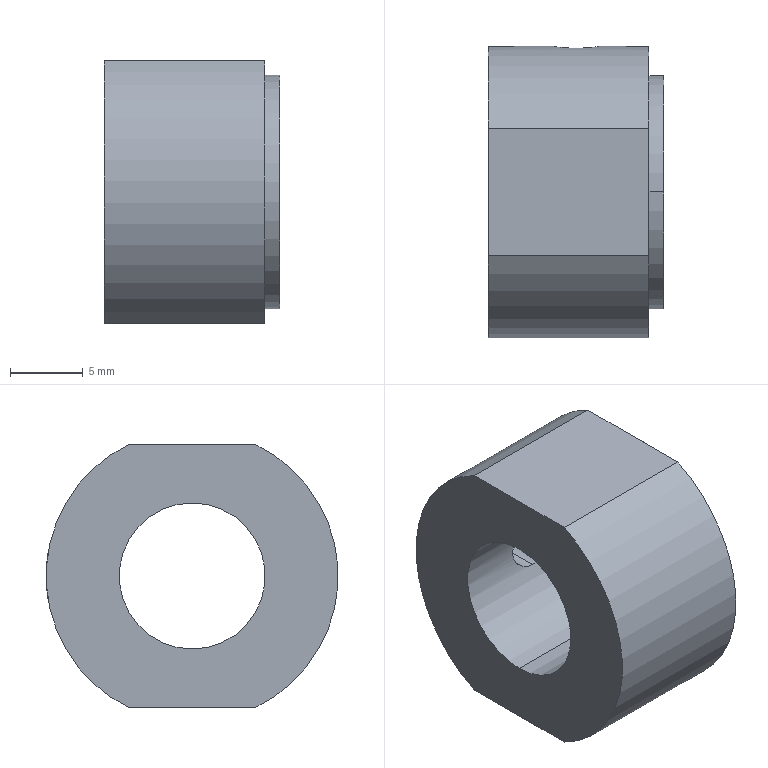Part | SolidWorks | features HoleWzd 1, ICE 1, Revolution 1 | 1 solid | 13 faces | box 12 x 20 x 18 mm | volume 2542 mm3 | cylinder 8 | plane 5 | commonest cylinder face diameters 3.3 x2 10 x2 16 x2 20 x2
STEP:
#1=CARTESIAN_POINT('',(6.,4.72,-1.65));
#2=VERTEX_POINT('',#1);
#3=CARTESIAN_POINT('',(6.,4.72,1.65));
#4=VERTEX_POINT('',#3);
#5=CARTESIAN_POINT('',(6.,4.72,-1.65));
#6=CARTESIAN_POINT('',(5.784,4.72,-1.65));
#7=CARTESIAN_POINT('',(5.565,4.736,-1.606));
#8=CARTESIAN_POINT('',(5.267,4.776,-1.482));
#9=CARTESIAN_POINT('',(5.17,4.791,-1.43));
#10=CARTESIAN_POINT('',(4.992,4.826,-1.311));
#11=CARTESIAN_POINT('',(4.91,4.844,-1.243));
#12=CARTESIAN_POINT('',(4.681,4.899,-1.014));
#13=CARTESIAN_POINT('',(4.56,4.934,-0.8345));
#14=CARTESIAN_POINT('',(4.435,4.972,-0.5335));
#15=CARTESIAN_POINT('',(4.403,4.983,-0.4304));
#16=CARTESIAN_POINT('',(4.361,4.996,-0.2186));
#17=CARTESIAN_POINT('',(4.35,5.,-0.1085));
#18=CARTESIAN_POINT('',(4.35,5.,0.1089));
#19=CARTESIAN_POINT('',(4.361,4.996,0.2166));
#20=CARTESIAN_POINT('',(4.403,4.983,0.4298));
#21=CARTESIAN_POINT('',(4.435,4.972,0.5348));
#22=CARTESIAN_POINT('',(4.559,4.934,0.8329));
#23=CARTESIAN_POINT('',(4.682,4.898,1.016));
#24=CARTESIAN_POINT('',(4.909,4.844,1.242));
#25=CARTESIAN_POINT('',(4.993,4.825,1.312));
#26=CARTESIAN_POINT('',(5.172,4.791,1.431));
#27=CARTESIAN_POINT('',(5.266,4.776,1.482));
#28=CARTESIAN_POINT('',(5.465,4.749,1.565));
#29=CARTESIAN_POINT('',(5.57,4.738,1.597));
#30=CARTESIAN_POINT('',(5.782,4.724,1.639));
#31=CARTESIAN_POINT('',(5.89,4.72,1.65));
#32=CARTESIAN_POINT('',(6.,4.72,1.65));
#33=B_SPLINE_CURVE_WITH_KNOTS('',3,(#5,#6,#7,#8,#9,#10,#11,#12,#13,#14,#15,#16,#17,#18,#19,#20,#21,#22,#23,#24,#25,#26,#27,#28,#29,#30,#31,#32),.UNSPECIFIED.,.F.,.F.,(4,2,2,2,2,2,2,2,2,2,2,2,2,4),(0.005195,0.005844,0.006169,0.006494,0.007143,0.007467,0.007792,0.008117,0.008441,0.009091,0.009415,0.00974,0.01006,0.01039),.UNSPECIFIED.);
#34=EDGE_CURVE('',#2,#4,#33,.T.);
#35=ORIENTED_EDGE('',*,*,#34,.F.);
#36=CARTESIAN_POINT('',(6.,9.863,-1.65));
#37=VERTEX_POINT('',#36);
#38=CARTESIAN_POINT('',(6.,10.,-1.65));
#39=DIRECTION('',(0.,1.,0.));
#40=VECTOR('',#39,1000.);
#41=LINE('',#38,#40);
#42=EDGE_CURVE('',#2,#37,#41,.T.);
#43=ORIENTED_EDGE('',*,*,#42,.T.);
#44=CARTESIAN_POINT('',(6.,9.863,1.65));
#45=VERTEX_POINT('',#44);
#46=CARTESIAN_POINT('',(6.,9.863,1.65));
#47=CARTESIAN_POINT('',(5.891,9.863,1.65));
#48=CARTESIAN_POINT('',(5.783,9.865,1.639));
#49=CARTESIAN_POINT('',(5.572,9.872,1.597));
#50=CARTESIAN_POINT('',(5.467,9.877,1.565));
#51=CARTESIAN_POINT('',(5.268,9.89,1.483));
#52=CARTESIAN_POINT('',(5.173,9.897,1.432));
#53=CARTESIAN_POINT('',(4.994,9.914,1.312));
#54=CARTESIAN_POINT('',(4.909,9.923,1.242));
#55=CARTESIAN_POINT('',(4.681,9.95,1.015));
#56=CARTESIAN_POINT('',(4.558,9.967,0.8307));
#57=CARTESIAN_POINT('',(4.394,9.993,0.4337));
#58=CARTESIAN_POINT('',(4.35,10.,0.2163));
#59=CARTESIAN_POINT('',(4.35,10.,-0.1072));
#60=CARTESIAN_POINT('',(4.361,9.998,-0.2168));
#61=CARTESIAN_POINT('',(4.403,9.991,-0.4285));
#62=CARTESIAN_POINT('',(4.434,9.986,-0.5315));
#63=CARTESIAN_POINT('',(4.558,9.967,-0.8315));
#64=CARTESIAN_POINT('',(4.68,9.95,-1.013));
#65=CARTESIAN_POINT('',(4.91,9.923,-1.244));
#66=CARTESIAN_POINT('',(4.993,9.914,-1.312));
#67=CARTESIAN_POINT('',(5.172,9.897,-1.431));
#68=CARTESIAN_POINT('',(5.268,9.89,-1.483));
#69=CARTESIAN_POINT('',(5.468,9.877,-1.566));
#70=CARTESIAN_POINT('',(5.571,9.872,-1.597));
#71=CARTESIAN_POINT('',(5.783,9.865,-1.639));
#72=CARTESIAN_POINT('',(5.892,9.863,-1.65));
#73=CARTESIAN_POINT('',(6.,9.863,-1.65));
#74=B_SPLINE_CURVE_WITH_KNOTS('',3,(#46,#47,#48,#49,#50,#51,#52,#53,#54,#55,#56,#57,#58,#59,#60,#61,#62,#63,#64,#65,#66,#67,#68,#69,#70,#71,#72,#73),.UNSPECIFIED.,.F.,.F.,(4,2,2,2,2,2,2,2,2,2,2,2,2,4),(0.,0.000323,0.0006459,0.0009689,0.001292,0.001938,0.002584,0.002907,0.00323,0.003876,0.004199,0.004522,0.004845,0.005167),.UNSPECIFIED.);
#75=EDGE_CURVE('',#45,#37,#74,.T.);
#76=ORIENTED_EDGE('',*,*,#75,.F.);
#77=CARTESIAN_POINT('',(6.,10.,1.65));
#78=DIRECTION('',(0.,1.,0.));
#79=VECTOR('',#78,1000.);
#80=LINE('',#77,#79);
#81=EDGE_CURVE('',#4,#45,#80,.T.);
#82=ORIENTED_EDGE('',*,*,#81,.F.);
#83=EDGE_LOOP('',(#35,#43,#76,#82));
#84=FACE_OUTER_BOUND('',#83,.T.);
#85=CARTESIAN_POINT('',(6.,10.,0.));
#86=DIRECTION('',(0.,1.,0.));
#87=DIRECTION('',(0.,0.,1.));
#88=AXIS2_PLACEMENT_3D('',#85,#86,#87);
#89=CYLINDRICAL_SURFACE('',#88,1.65);
#90=ADVANCED_FACE('',(#84),#89,.F.);
#91=CARTESIAN_POINT('',(12.,0.,8.));
#92=VERTEX_POINT('',#91);
#93=CARTESIAN_POINT('',(12.,0.,-8.));
#94=VERTEX_POINT('',#93);
#95=CARTESIAN_POINT('',(12.,0.,0.));
#96=DIRECTION('',(-1.,0.,0.));
#97=DIRECTION('',(0.,0.,1.));
#98=AXIS2_PLACEMENT_3D('',#95,#96,#97);
#99=CIRCLE('',#98,8.);
#100=EDGE_CURVE('',#92,#94,#99,.T.);
#101=ORIENTED_EDGE('',*,*,#100,.T.);
#102=CARTESIAN_POINT('',(11.,0.,-8.));
#103=VERTEX_POINT('',#102);
#104=CARTESIAN_POINT('',(0.,0.,-8.));
#105=DIRECTION('',(-1.,0.,0.));
#106=VECTOR('',#105,1000.);
#107=LINE('',#104,#106);
#108=EDGE_CURVE('',#94,#103,#107,.T.);
#109=ORIENTED_EDGE('',*,*,#108,.T.);
#110=CARTESIAN_POINT('',(11.,0.,8.));
#111=VERTEX_POINT('',#110);
#112=CARTESIAN_POINT('',(11.,0.,0.));
#113=DIRECTION('',(-1.,0.,0.));
#114=DIRECTION('',(0.,0.,1.));
#115=AXIS2_PLACEMENT_3D('',#112,#113,#114);
#116=CIRCLE('',#115,8.);
#117=EDGE_CURVE('',#111,#103,#116,.T.);
#118=ORIENTED_EDGE('',*,*,#117,.F.);
#119=CARTESIAN_POINT('',(0.,0.,8.));
#120=DIRECTION('',(-1.,0.,0.));
#121=VECTOR('',#120,1000.);
#122=LINE('',#119,#121);
#123=EDGE_CURVE('',#92,#111,#122,.T.);
#124=ORIENTED_EDGE('',*,*,#123,.F.);
#125=EDGE_LOOP('',(#101,#109,#118,#124));
#126=FACE_OUTER_BOUND('',#125,.T.);
#127=CARTESIAN_POINT('',(0.,0.,0.));
#128=DIRECTION('',(-1.,0.,0.));
#129=DIRECTION('',(0.,0.,1.));
#130=AXIS2_PLACEMENT_3D('',#127,#128,#129);
#131=CYLINDRICAL_SURFACE('',#130,8.);
#132=ADVANCED_FACE('',(#126),#131,.T.);
#133=CARTESIAN_POINT('',(12.,0.,-5.));
#134=VERTEX_POINT('',#133);
#135=CARTESIAN_POINT('',(12.,0.,5.));
#136=VERTEX_POINT('',#135);
#137=CARTESIAN_POINT('',(12.,0.,0.));
#138=DIRECTION('',(-1.,0.,0.));
#139=DIRECTION('',(0.,0.,1.));
#140=AXIS2_PLACEMENT_3D('',#137,#138,#139);
#141=CIRCLE('',#140,5.);
#142=EDGE_CURVE('',#134,#136,#141,.T.);
#143=ORIENTED_EDGE('',*,*,#142,.F.);
#144=CARTESIAN_POINT('',(0.,0.,-5.));
#145=VERTEX_POINT('',#144);
#146=CARTESIAN_POINT('',(0.,0.,-5.));
#147=DIRECTION('',(-1.,0.,0.));
#148=VECTOR('',#147,1000.);
#149=LINE('',#146,#148);
#150=EDGE_CURVE('',#134,#145,#149,.T.);
#151=ORIENTED_EDGE('',*,*,#150,.T.);
#152=CARTESIAN_POINT('',(0.,0.,5.));
#153=VERTEX_POINT('',#152);
#154=CARTESIAN_POINT('',(0.,0.,0.));
#155=DIRECTION('',(-1.,0.,0.));
#156=DIRECTION('',(0.,0.,1.));
#157=AXIS2_PLACEMENT_3D('',#154,#155,#156);
#158=CIRCLE('',#157,5.);
#159=EDGE_CURVE('',#145,#153,#158,.T.);
#160=ORIENTED_EDGE('',*,*,#159,.T.);
#161=CARTESIAN_POINT('',(0.,0.,5.));
#162=DIRECTION('',(-1.,0.,0.));
#163=VECTOR('',#162,1000.);
#164=LINE('',#161,#163);
#165=EDGE_CURVE('',#136,#153,#164,.T.);
#166=ORIENTED_EDGE('',*,*,#165,.F.);
#167=EDGE_LOOP('',(#143,#151,#160,#166));
#168=FACE_OUTER_BOUND('',#167,.T.);
#169=CARTESIAN_POINT('',(0.,0.,0.));
#170=DIRECTION('',(-1.,0.,0.));
#171=DIRECTION('',(0.,0.,1.));
#172=AXIS2_PLACEMENT_3D('',#169,#170,#171);
#173=CYLINDRICAL_SURFACE('',#172,5.);
#174=ADVANCED_FACE('',(#168),#173,.F.);
#175=CARTESIAN_POINT('',(0.,0.,0.));
#176=DIRECTION('',(-1.,0.,0.));
#177=DIRECTION('',(0.,0.,1.));
#178=AXIS2_PLACEMENT_3D('',#175,#176,#177);
#179=CIRCLE('',#178,5.);
#180=EDGE_CURVE('',#153,#145,#179,.T.);
#181=ORIENTED_EDGE('',*,*,#180,.F.);
#182=ORIENTED_EDGE('',*,*,#159,.F.);
#183=EDGE_LOOP('',(#181,#182));
#184=FACE_BOUND('',#183,.T.);
#185=CARTESIAN_POINT('',(0.,-4.359,9.));
#186=VERTEX_POINT('',#185);
#187=CARTESIAN_POINT('',(0.,4.359,9.));
#188=VERTEX_POINT('',#187);
#189=CARTESIAN_POINT('',(0.,12.5,9.));
#190=DIRECTION('',(0.,1.,0.));
#191=VECTOR('',#190,1000.);
#192=LINE('',#189,#191);
#193=EDGE_CURVE('',#186,#188,#192,.T.);
#194=ORIENTED_EDGE('',*,*,#193,.T.);
#195=CARTESIAN_POINT('',(0.,4.359,-9.));
#196=VERTEX_POINT('',#195);
#197=CARTESIAN_POINT('',(0.,0.,0.));
#198=DIRECTION('',(-1.,0.,0.));
#199=DIRECTION('',(0.,0.,1.));
#200=AXIS2_PLACEMENT_3D('',#197,#198,#199);
#201=CIRCLE('',#200,10.);
#202=EDGE_CURVE('',#188,#196,#201,.T.);
#203=ORIENTED_EDGE('',*,*,#202,.T.);
#204=CARTESIAN_POINT('',(0.,-4.359,-9.));
#205=VERTEX_POINT('',#204);
#206=CARTESIAN_POINT('',(0.,12.5,-9.));
#207=DIRECTION('',(0.,-1.,0.));
#208=VECTOR('',#207,1000.);
#209=LINE('',#206,#208);
#210=EDGE_CURVE('',#196,#205,#209,.T.);
#211=ORIENTED_EDGE('',*,*,#210,.T.);
#212=CARTESIAN_POINT('',(0.,0.,0.));
#213=DIRECTION('',(-1.,0.,0.));
#214=DIRECTION('',(0.,0.,1.));
#215=AXIS2_PLACEMENT_3D('',#212,#213,#214);
#216=CIRCLE('',#215,10.);
#217=EDGE_CURVE('',#205,#186,#216,.T.);
#218=ORIENTED_EDGE('',*,*,#217,.T.);
#219=EDGE_LOOP('',(#194,#203,#211,#218));
#220=FACE_OUTER_BOUND('',#219,.T.);
#221=CARTESIAN_POINT('',(0.,5.,0.));
#222=DIRECTION('',(1.,0.,0.));
#223=DIRECTION('',(0.,0.,-1.));
#224=AXIS2_PLACEMENT_3D('',#221,#222,#223);
#225=PLANE('',#224);
#226=ADVANCED_FACE('',(#184,#220),#225,.F.);
#227=ORIENTED_EDGE('',*,*,#75,.T.);
#228=CARTESIAN_POINT('',(6.,9.863,-1.65));
#229=CARTESIAN_POINT('',(6.216,9.863,-1.65));
#230=CARTESIAN_POINT('',(6.433,9.87,-1.607));
#231=CARTESIAN_POINT('',(6.83,9.896,-1.442));
#232=CARTESIAN_POINT('',(7.014,9.914,-1.319));
#233=CARTESIAN_POINT('',(7.242,9.941,-1.091));
#234=CARTESIAN_POINT('',(7.312,9.95,-1.007));
#235=CARTESIAN_POINT('',(7.431,9.966,-0.8279));
#236=CARTESIAN_POINT('',(7.482,9.974,-0.7333));
#237=CARTESIAN_POINT('',(7.607,9.993,-0.4334));
#238=CARTESIAN_POINT('',(7.65,10.,-0.219));
#239=CARTESIAN_POINT('',(7.65,10.,0.108));
#240=CARTESIAN_POINT('',(7.639,9.998,0.2153));
#241=CARTESIAN_POINT('',(7.598,9.991,0.4265));
#242=CARTESIAN_POINT('',(7.566,9.986,0.5316));
#243=CARTESIAN_POINT('',(7.483,9.974,0.7311));
#244=CARTESIAN_POINT('',(7.433,9.966,0.8259));
#245=CARTESIAN_POINT('',(7.313,9.95,1.005));
#246=CARTESIAN_POINT('',(7.243,9.941,1.09));
#247=CARTESIAN_POINT('',(7.016,9.914,1.318));
#248=CARTESIAN_POINT('',(6.832,9.896,1.441));
#249=CARTESIAN_POINT('',(6.435,9.871,1.606));
#250=CARTESIAN_POINT('',(6.218,9.863,1.65));
#251=CARTESIAN_POINT('',(6.,9.863,1.65));
#252=B_SPLINE_CURVE_WITH_KNOTS('',3,(#228,#229,#230,#231,#232,#233,#234,#235,#236,#237,#238,#239,#240,#241,#242,#243,#244,#245,#246,#247,#248,#249,#250,#251),.UNSPECIFIED.,.F.,.F.,(4,2,2,2,2,2,2,2,2,2,2,4),(0.005167,0.005813,0.006459,0.006782,0.007105,0.007751,0.008073,0.008396,0.008719,0.009042,0.009688,0.01033),.UNSPECIFIED.);
#253=EDGE_CURVE('',#37,#45,#252,.T.);
#254=ORIENTED_EDGE('',*,*,#253,.T.);
#255=EDGE_LOOP('',(#227,#254));
#256=FACE_BOUND('',#255,.T.);
#257=CARTESIAN_POINT('',(11.,4.359,9.));
#258=VERTEX_POINT('',#257);
#259=CARTESIAN_POINT('',(0.,4.359,9.));
#260=DIRECTION('',(-1.,0.,0.));
#261=VECTOR('',#260,1000.);
#262=LINE('',#259,#261);
#263=EDGE_CURVE('',#258,#188,#262,.T.);
#264=ORIENTED_EDGE('',*,*,#263,.F.);
#265=CARTESIAN_POINT('',(11.,4.359,-9.));
#266=VERTEX_POINT('',#265);
#267=CARTESIAN_POINT('',(11.,0.,0.));
#268=DIRECTION('',(-1.,0.,0.));
#269=DIRECTION('',(0.,0.,1.));
#270=AXIS2_PLACEMENT_3D('',#267,#268,#269);
#271=CIRCLE('',#270,10.);
#272=EDGE_CURVE('',#258,#266,#271,.T.);
#273=ORIENTED_EDGE('',*,*,#272,.T.);
#274=CARTESIAN_POINT('',(0.,4.359,-9.));
#275=DIRECTION('',(1.,0.,0.));
#276=VECTOR('',#275,1000.);
#277=LINE('',#274,#276);
#278=EDGE_CURVE('',#196,#266,#277,.T.);
#279=ORIENTED_EDGE('',*,*,#278,.F.);
#280=ORIENTED_EDGE('',*,*,#202,.F.);
#281=EDGE_LOOP('',(#264,#273,#279,#280));
#282=FACE_OUTER_BOUND('',#281,.T.);
#283=CARTESIAN_POINT('',(0.,0.,0.));
#284=DIRECTION('',(-1.,0.,0.));
#285=DIRECTION('',(0.,0.,1.));
#286=AXIS2_PLACEMENT_3D('',#283,#284,#285);
#287=CYLINDRICAL_SURFACE('',#286,10.);
#288=ADVANCED_FACE('',(#256,#282),#287,.T.);
#289=CARTESIAN_POINT('',(11.,-4.359,9.));
#290=VERTEX_POINT('',#289);
#291=CARTESIAN_POINT('',(0.,-4.359,9.));
#292=DIRECTION('',(1.,0.,0.));
#293=VECTOR('',#292,1000.);
#294=LINE('',#291,#293);
#295=EDGE_CURVE('',#186,#290,#294,.T.);
#296=ORIENTED_EDGE('',*,*,#295,.F.);
#297=ORIENTED_EDGE('',*,*,#217,.F.);
#298=CARTESIAN_POINT('',(11.,-4.359,-9.));
#299=VERTEX_POINT('',#298);
#300=CARTESIAN_POINT('',(0.,-4.359,-9.));
#301=DIRECTION('',(-1.,0.,0.));
#302=VECTOR('',#301,1000.);
#303=LINE('',#300,#302);
#304=EDGE_CURVE('',#299,#205,#303,.T.);
#305=ORIENTED_EDGE('',*,*,#304,.F.);
#306=CARTESIAN_POINT('',(11.,0.,0.));
#307=DIRECTION('',(-1.,0.,0.));
#308=DIRECTION('',(0.,0.,1.));
#309=AXIS2_PLACEMENT_3D('',#306,#307,#308);
#310=CIRCLE('',#309,10.);
#311=EDGE_CURVE('',#299,#290,#310,.T.);
#312=ORIENTED_EDGE('',*,*,#311,.T.);
#313=EDGE_LOOP('',(#296,#297,#305,#312));
#314=FACE_OUTER_BOUND('',#313,.T.);
#315=CARTESIAN_POINT('',(0.,0.,0.));
#316=DIRECTION('',(-1.,0.,0.));
#317=DIRECTION('',(0.,0.,1.));
#318=AXIS2_PLACEMENT_3D('',#315,#316,#317);
#319=CYLINDRICAL_SURFACE('',#318,10.);
#320=ADVANCED_FACE('',(#314),#319,.T.);
#321=ORIENTED_EDGE('',*,*,#117,.T.);
#322=CARTESIAN_POINT('',(11.,0.,0.));
#323=DIRECTION('',(-1.,0.,0.));
#324=DIRECTION('',(0.,0.,1.));
#325=AXIS2_PLACEMENT_3D('',#322,#323,#324);
#326=CIRCLE('',#325,8.);
#327=EDGE_CURVE('',#103,#111,#326,.T.);
#328=ORIENTED_EDGE('',*,*,#327,.T.);
#329=EDGE_LOOP('',(#321,#328));
#330=FACE_BOUND('',#329,.T.);
#331=CARTESIAN_POINT('',(11.,10.,9.));
#332=DIRECTION('',(0.,1.,0.));
#333=VECTOR('',#332,1000.);
#334=LINE('',#331,#333);
#335=EDGE_CURVE('',#290,#258,#334,.T.);
#336=ORIENTED_EDGE('',*,*,#335,.F.);
#337=ORIENTED_EDGE('',*,*,#311,.F.);
#338=CARTESIAN_POINT('',(11.,10.,-9.));
#339=DIRECTION('',(0.,-1.,0.));
#340=VECTOR('',#339,1000.);
#341=LINE('',#338,#340);
#342=EDGE_CURVE('',#266,#299,#341,.T.);
#343=ORIENTED_EDGE('',*,*,#342,.F.);
#344=ORIENTED_EDGE('',*,*,#272,.F.);
#345=EDGE_LOOP('',(#336,#337,#343,#344));
#346=FACE_OUTER_BOUND('',#345,.T.);
#347=CARTESIAN_POINT('',(11.,10.,0.));
#348=DIRECTION('',(-1.,0.,0.));
#349=DIRECTION('',(0.,0.,1.));
#350=AXIS2_PLACEMENT_3D('',#347,#348,#349);
#351=PLANE('',#350);
#352=ADVANCED_FACE('',(#330,#346),#351,.F.);
#353=ORIENTED_EDGE('',*,*,#150,.F.);
#354=CARTESIAN_POINT('',(12.,0.,0.));
#355=DIRECTION('',(-1.,0.,0.));
#356=DIRECTION('',(0.,0.,1.));
#357=AXIS2_PLACEMENT_3D('',#354,#355,#356);
#358=CIRCLE('',#357,5.);
#359=EDGE_CURVE('',#136,#134,#358,.T.);
#360=ORIENTED_EDGE('',*,*,#359,.F.);
#361=ORIENTED_EDGE('',*,*,#165,.T.);
#362=ORIENTED_EDGE('',*,*,#180,.T.);
#363=EDGE_LOOP('',(#353,#360,#361,#362));
#364=FACE_OUTER_BOUND('',#363,.T.);
#365=CARTESIAN_POINT('',(6.,4.72,1.65));
#366=CARTESIAN_POINT('',(6.11,4.72,1.65));
#367=CARTESIAN_POINT('',(6.218,4.724,1.639));
#368=CARTESIAN_POINT('',(6.43,4.738,1.597));
#369=CARTESIAN_POINT('',(6.535,4.749,1.565));
#370=CARTESIAN_POINT('',(6.734,4.776,1.482));
#371=CARTESIAN_POINT('',(6.829,4.791,1.431));
#372=CARTESIAN_POINT('',(7.007,4.825,1.311));
#373=CARTESIAN_POINT('',(7.091,4.844,1.242));
#374=CARTESIAN_POINT('',(7.318,4.898,1.015));
#375=CARTESIAN_POINT('',(7.441,4.934,0.8326));
#376=CARTESIAN_POINT('',(7.565,4.972,0.5351));
#377=CARTESIAN_POINT('',(7.597,4.983,0.4303));
#378=CARTESIAN_POINT('',(7.639,4.996,0.2169));
#379=CARTESIAN_POINT('',(7.65,5.,0.1093));
#380=CARTESIAN_POINT('',(7.65,5.,-0.1078));
#381=CARTESIAN_POINT('',(7.639,4.996,-0.218));
#382=CARTESIAN_POINT('',(7.597,4.983,-0.4303));
#383=CARTESIAN_POINT('',(7.565,4.972,-0.5336));
#384=CARTESIAN_POINT('',(7.44,4.934,-0.8348));
#385=CARTESIAN_POINT('',(7.318,4.898,-1.016));
#386=CARTESIAN_POINT('',(7.09,4.844,-1.243));
#387=CARTESIAN_POINT('',(7.007,4.825,-1.311));
#388=CARTESIAN_POINT('',(6.829,4.791,-1.431));
#389=CARTESIAN_POINT('',(6.733,4.775,-1.482));
#390=CARTESIAN_POINT('',(6.534,4.749,-1.565));
#391=CARTESIAN_POINT('',(6.431,4.738,-1.596));
#392=CARTESIAN_POINT('',(6.218,4.724,-1.639));
#393=CARTESIAN_POINT('',(6.108,4.72,-1.65));
#394=CARTESIAN_POINT('',(6.,4.72,-1.65));
#395=B_SPLINE_CURVE_WITH_KNOTS('',3,(#365,#366,#367,#368,#369,#370,#371,#372,#373,#374,#375,#376,#377,#378,#379,#380,#381,#382,#383,#384,#385,#386,#387,#388,#389,#390,#391,#392,#393,#394),.UNSPECIFIED.,.F.,.F.,(4,2,2,2,2,2,2,2,2,2,2,2,2,2,4),(0.,0.0003247,0.0006494,0.0009741,0.001299,0.001948,0.002273,0.002598,0.002922,0.003247,0.003896,0.004221,0.004546,0.00487,0.005195),.UNSPECIFIED.);
#396=EDGE_CURVE('',#4,#2,#395,.T.);
#397=ORIENTED_EDGE('',*,*,#396,.T.);
#398=ORIENTED_EDGE('',*,*,#34,.T.);
#399=EDGE_LOOP('',(#397,#398));
#400=FACE_BOUND('',#399,.T.);
#401=CARTESIAN_POINT('',(0.,0.,0.));
#402=DIRECTION('',(-1.,0.,0.));
#403=DIRECTION('',(0.,0.,1.));
#404=AXIS2_PLACEMENT_3D('',#401,#402,#403);
#405=CYLINDRICAL_SURFACE('',#404,5.);
#406=ADVANCED_FACE('',(#364,#400),#405,.F.);
#407=ORIENTED_EDGE('',*,*,#108,.F.);
#408=CARTESIAN_POINT('',(12.,0.,0.));
#409=DIRECTION('',(-1.,0.,0.));
#410=DIRECTION('',(0.,0.,1.));
#411=AXIS2_PLACEMENT_3D('',#408,#409,#410);
#412=CIRCLE('',#411,8.);
#413=EDGE_CURVE('',#94,#92,#412,.T.);
#414=ORIENTED_EDGE('',*,*,#413,.T.);
#415=ORIENTED_EDGE('',*,*,#123,.T.);
#416=ORIENTED_EDGE('',*,*,#327,.F.);
#417=EDGE_LOOP('',(#407,#414,#415,#416));
#418=FACE_OUTER_BOUND('',#417,.T.);
#419=CARTESIAN_POINT('',(0.,0.,0.));
#420=DIRECTION('',(-1.,0.,0.));
#421=DIRECTION('',(0.,0.,1.));
#422=AXIS2_PLACEMENT_3D('',#419,#420,#421);
#423=CYLINDRICAL_SURFACE('',#422,8.);
#424=ADVANCED_FACE('',(#418),#423,.T.);
#425=ORIENTED_EDGE('',*,*,#100,.F.);
#426=ORIENTED_EDGE('',*,*,#413,.F.);
#427=EDGE_LOOP('',(#425,#426));
#428=FACE_OUTER_BOUND('',#427,.T.);
#429=ORIENTED_EDGE('',*,*,#359,.T.);
#430=ORIENTED_EDGE('',*,*,#142,.T.);
#431=EDGE_LOOP('',(#429,#430));
#432=FACE_BOUND('',#431,.T.);
#433=CARTESIAN_POINT('',(12.,8.,0.));
#434=DIRECTION('',(-1.,0.,0.));
#435=DIRECTION('',(0.,0.,1.));
#436=AXIS2_PLACEMENT_3D('',#433,#434,#435);
#437=PLANE('',#436);
#438=ADVANCED_FACE('',(#428,#432),#437,.F.);
#439=ORIENTED_EDGE('',*,*,#304,.T.);
#440=ORIENTED_EDGE('',*,*,#210,.F.);
#441=ORIENTED_EDGE('',*,*,#278,.T.);
#442=ORIENTED_EDGE('',*,*,#342,.T.);
#443=EDGE_LOOP('',(#439,#440,#441,#442));
#444=FACE_OUTER_BOUND('',#443,.T.);
#445=CARTESIAN_POINT('',(12.,12.5,-9.));
#446=DIRECTION('',(0.,0.,-1.));
#447=DIRECTION('',(0.,1.,0.));
#448=AXIS2_PLACEMENT_3D('',#445,#446,#447);
#449=PLANE('',#448);
#450=ADVANCED_FACE('',(#444),#449,.T.);
#451=ORIENTED_EDGE('',*,*,#263,.T.);
#452=ORIENTED_EDGE('',*,*,#193,.F.);
#453=ORIENTED_EDGE('',*,*,#295,.T.);
#454=ORIENTED_EDGE('',*,*,#335,.T.);
#455=EDGE_LOOP('',(#451,#452,#453,#454));
#456=FACE_OUTER_BOUND('',#455,.T.);
#457=CARTESIAN_POINT('',(12.,12.5,9.));
#458=DIRECTION('',(0.,0.,1.));
#459=DIRECTION('',(0.,-1.,0.));
#460=AXIS2_PLACEMENT_3D('',#457,#458,#459);
#461=PLANE('',#460);
#462=ADVANCED_FACE('',(#456),#461,.T.);
#463=ORIENTED_EDGE('',*,*,#42,.F.);
#464=ORIENTED_EDGE('',*,*,#396,.F.);
#465=ORIENTED_EDGE('',*,*,#81,.T.);
#466=ORIENTED_EDGE('',*,*,#253,.F.);
#467=EDGE_LOOP('',(#463,#464,#465,#466));
#468=FACE_OUTER_BOUND('',#467,.T.);
#469=CARTESIAN_POINT('',(6.,10.,0.));
#470=DIRECTION('',(0.,1.,0.));
#471=DIRECTION('',(0.,0.,1.));
#472=AXIS2_PLACEMENT_3D('',#469,#470,#471);
#473=CYLINDRICAL_SURFACE('',#472,1.65);
#474=ADVANCED_FACE('',(#468),#473,.F.);
#475=CLOSED_SHELL('',(#90,#132,#174,#226,#288,#320,#352,#406,#424,#438,#450,#462,#474));
#476=MANIFOLD_SOLID_BREP('',#475);
#477=CARTESIAN_POINT('',(0.,0.,0.));
#478=DIRECTION('',(0.,0.,1.));
#479=DIRECTION('',(1.,0.,0.));
#480=AXIS2_PLACEMENT_3D('',#477,#478,#479);
#481=(LENGTH_UNIT()NAMED_UNIT(*)SI_UNIT(.MILLI.,.METRE.));
#482=UNCERTAINTY_MEASURE_WITH_UNIT(LENGTH_MEASURE(0.00001),#481,'','');
#483=(NAMED_UNIT(*)PLANE_ANGLE_UNIT()SI_UNIT($,.RADIAN.));
#484=(NAMED_UNIT(*)SI_UNIT($,.STERADIAN.)SOLID_ANGLE_UNIT());
#485=(GEOMETRIC_REPRESENTATION_CONTEXT(3)GLOBAL_UNCERTAINTY_ASSIGNED_CONTEXT((#482))GLOBAL_UNIT_ASSIGNED_CONTEXT((#481,#483,#484))REPRESENTATION_CONTEXT('',''));
#486=ADVANCED_BREP_SHAPE_REPRESENTATION('',(#476,#480),#485);